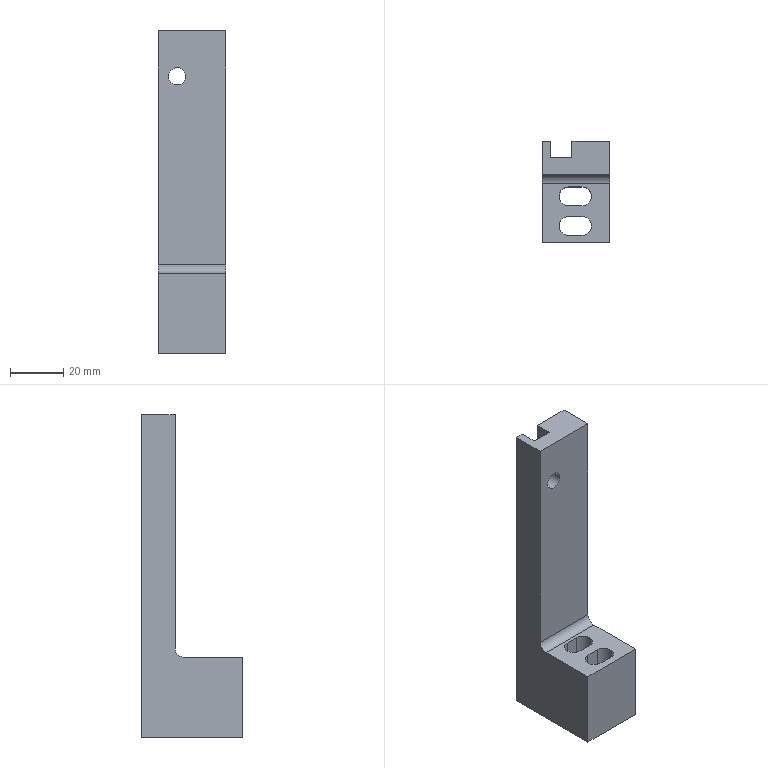Part | STEP file | 1_id1446_x_t | 1 solid | 23 faces | box 25.4 x 38.1 x 121.275 mm | volume 47668 mm3 | plane 16 | cylinder 7 | commonest cylinder face diameters 7.144 x4 6.5 x2 6.35 x1